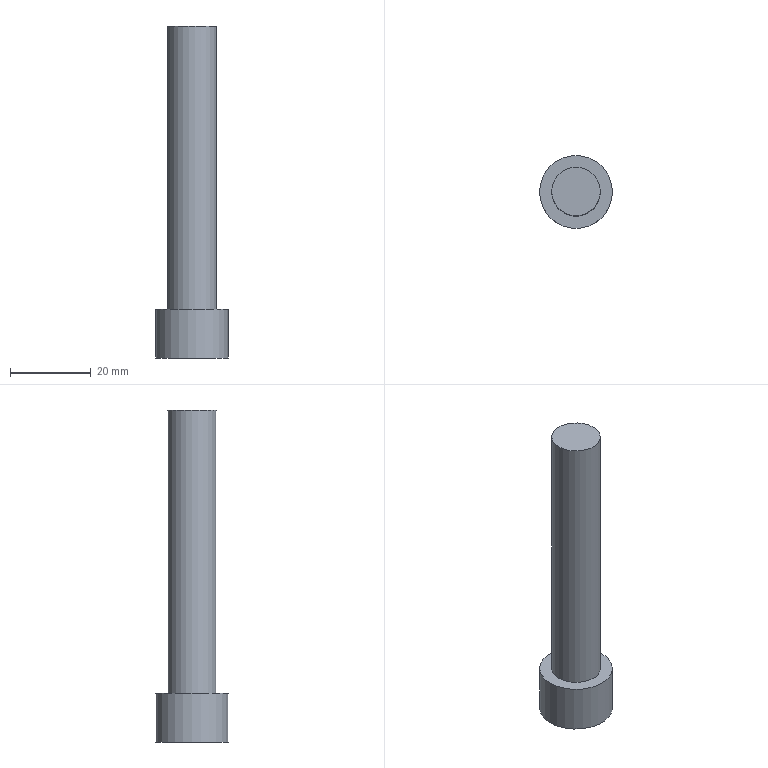Part | NX | features solid 2 | 1 solid | 12 faces | box 18 x 18 x 82 mm | volume 10451 mm3 | plane 10 | cylinder 2 | commonest cylinder face diameters 12 x1 18 x1
STEP:
#1=CARTESIAN_POINT('',(-264.,-305.,267.));
#2=VERTEX_POINT('',#1);
#3=CARTESIAN_POINT('',(-270.,-305.,267.));
#4=DIRECTION('',(0.,0.,1.));
#5=DIRECTION('',(1.,0.,0.));
#6=AXIS2_PLACEMENT_3D('',#3,#4,#5);
#7=CIRCLE('',#6,6.);
#8=EDGE_CURVE('',#2,#2,#7,.T.);
#9=ORIENTED_EDGE('',*,*,#8,.T.);
#10=EDGE_LOOP('',(#9));
#11=FACE_BOUND('',#10,.T.);
#12=CARTESIAN_POINT('',(-264.,-305.,337.));
#13=VERTEX_POINT('',#12);
#14=CARTESIAN_POINT('',(-270.,-305.,337.));
#15=DIRECTION('',(0.,0.,1.));
#16=DIRECTION('',(1.,0.,0.));
#17=AXIS2_PLACEMENT_3D('',#14,#15,#16);
#18=CIRCLE('',#17,6.);
#19=EDGE_CURVE('',#13,#13,#18,.T.);
#20=ORIENTED_EDGE('',*,*,#19,.F.);
#21=EDGE_LOOP('',(#20));
#22=FACE_BOUND('',#21,.T.);
#23=CARTESIAN_POINT('',(-270.,-305.,337.));
#24=DIRECTION('',(0.,0.,-1.));
#25=DIRECTION('',(-1.,0.,0.));
#26=AXIS2_PLACEMENT_3D('',#23,#24,#25);
#27=CYLINDRICAL_SURFACE('',#26,6.);
#28=ADVANCED_FACE('',(#11,#22),#27,.T.);
#29=ORIENTED_EDGE('',*,*,#19,.T.);
#30=EDGE_LOOP('',(#29));
#31=FACE_BOUND('',#30,.T.);
#32=CARTESIAN_POINT('',(-270.,-305.,337.));
#33=DIRECTION('',(0.,0.,1.));
#34=DIRECTION('',(1.,0.,0.));
#35=AXIS2_PLACEMENT_3D('',#32,#33,#34);
#36=PLANE('',#35);
#37=ADVANCED_FACE('',(#31),#36,.T.);
#38=CARTESIAN_POINT('',(-261.,-305.,267.));
#39=VERTEX_POINT('',#38);
#40=CARTESIAN_POINT('',(-270.,-305.,267.));
#41=DIRECTION('',(0.,0.,1.));
#42=DIRECTION('',(1.,0.,0.));
#43=AXIS2_PLACEMENT_3D('',#40,#41,#42);
#44=CIRCLE('',#43,9.);
#45=EDGE_CURVE('',#39,#39,#44,.T.);
#46=ORIENTED_EDGE('',*,*,#45,.T.);
#47=EDGE_LOOP('',(#46));
#48=FACE_BOUND('',#47,.T.);
#49=ORIENTED_EDGE('',*,*,#8,.F.);
#50=EDGE_LOOP('',(#49));
#51=FACE_BOUND('',#50,.T.);
#52=CARTESIAN_POINT('',(-270.,-305.,267.));
#53=DIRECTION('',(0.,0.,1.));
#54=DIRECTION('',(1.,0.,0.));
#55=AXIS2_PLACEMENT_3D('',#52,#53,#54);
#56=PLANE('',#55);
#57=ADVANCED_FACE('',(#48,#51),#56,.T.);
#58=CARTESIAN_POINT('',(-261.,-305.,255.));
#59=VERTEX_POINT('',#58);
#60=CARTESIAN_POINT('',(-270.,-305.,255.));
#61=DIRECTION('',(0.,0.,1.));
#62=DIRECTION('',(1.,0.,0.));
#63=AXIS2_PLACEMENT_3D('',#60,#61,#62);
#64=CIRCLE('',#63,9.);
#65=EDGE_CURVE('',#59,#59,#64,.T.);
#66=ORIENTED_EDGE('',*,*,#65,.T.);
#67=EDGE_LOOP('',(#66));
#68=FACE_BOUND('',#67,.T.);
#69=ORIENTED_EDGE('',*,*,#45,.F.);
#70=EDGE_LOOP('',(#69));
#71=FACE_BOUND('',#70,.T.);
#72=CARTESIAN_POINT('',(-270.,-305.,255.));
#73=DIRECTION('',(0.,0.,1.));
#74=DIRECTION('',(1.,0.,0.));
#75=AXIS2_PLACEMENT_3D('',#72,#73,#74);
#76=CYLINDRICAL_SURFACE('',#75,9.);
#77=ADVANCED_FACE('',(#68,#71),#76,.T.);
#78=CARTESIAN_POINT('',(-265.,-302.113,255.));
#79=VERTEX_POINT('',#78);
#80=CARTESIAN_POINT('',(-270.,-299.226,255.));
#81=VERTEX_POINT('',#80);
#82=CARTESIAN_POINT('',(-267.5,-300.67,255.));
#83=DIRECTION('',(-0.866,0.5,0.));
#84=VECTOR('',#83,1000.);
#85=LINE('',#82,#84);
#86=EDGE_CURVE('',#79,#81,#85,.T.);
#87=ORIENTED_EDGE('',*,*,#86,.T.);
#88=CARTESIAN_POINT('',(-275.,-302.113,255.));
#89=VERTEX_POINT('',#88);
#90=CARTESIAN_POINT('',(-272.5,-300.67,255.));
#91=DIRECTION('',(-0.866,-0.5,0.));
#92=VECTOR('',#91,1000.);
#93=LINE('',#90,#92);
#94=EDGE_CURVE('',#81,#89,#93,.T.);
#95=ORIENTED_EDGE('',*,*,#94,.T.);
#96=CARTESIAN_POINT('',(-275.,-307.887,255.));
#97=VERTEX_POINT('',#96);
#98=CARTESIAN_POINT('',(-275.,-305.,255.));
#99=DIRECTION('',(0.,-1.,0.));
#100=VECTOR('',#99,1000.);
#101=LINE('',#98,#100);
#102=EDGE_CURVE('',#89,#97,#101,.T.);
#103=ORIENTED_EDGE('',*,*,#102,.T.);
#104=CARTESIAN_POINT('',(-270.,-310.774,255.));
#105=VERTEX_POINT('',#104);
#106=CARTESIAN_POINT('',(-272.5,-309.33,255.));
#107=DIRECTION('',(0.866,-0.5,0.));
#108=VECTOR('',#107,1000.);
#109=LINE('',#106,#108);
#110=EDGE_CURVE('',#97,#105,#109,.T.);
#111=ORIENTED_EDGE('',*,*,#110,.T.);
#112=CARTESIAN_POINT('',(-265.,-307.887,255.));
#113=VERTEX_POINT('',#112);
#114=CARTESIAN_POINT('',(-267.5,-309.33,255.));
#115=DIRECTION('',(0.866,0.5,0.));
#116=VECTOR('',#115,1000.);
#117=LINE('',#114,#116);
#118=EDGE_CURVE('',#105,#113,#117,.T.);
#119=ORIENTED_EDGE('',*,*,#118,.T.);
#120=CARTESIAN_POINT('',(-265.,-305.,255.));
#121=DIRECTION('',(0.,1.,0.));
#122=VECTOR('',#121,1000.);
#123=LINE('',#120,#122);
#124=EDGE_CURVE('',#113,#79,#123,.T.);
#125=ORIENTED_EDGE('',*,*,#124,.T.);
#126=EDGE_LOOP('',(#87,#95,#103,#111,#119,#125));
#127=FACE_BOUND('',#126,.T.);
#128=ORIENTED_EDGE('',*,*,#65,.F.);
#129=EDGE_LOOP('',(#128));
#130=FACE_BOUND('',#129,.T.);
#131=CARTESIAN_POINT('',(-270.,-305.,255.));
#132=DIRECTION('',(0.,0.,1.));
#133=DIRECTION('',(1.,0.,0.));
#134=AXIS2_PLACEMENT_3D('',#131,#132,#133);
#135=PLANE('',#134);
#136=ADVANCED_FACE('',(#127,#130),#135,.F.);
#137=CARTESIAN_POINT('',(-270.,-299.226,261.));
#138=VERTEX_POINT('',#137);
#139=CARTESIAN_POINT('',(-270.,-299.226,241.));
#140=DIRECTION('',(0.,0.,1.));
#141=VECTOR('',#140,1000.);
#142=LINE('',#139,#141);
#143=EDGE_CURVE('',#81,#138,#142,.T.);
#144=ORIENTED_EDGE('',*,*,#143,.T.);
#145=CARTESIAN_POINT('',(-275.,-302.113,261.));
#146=VERTEX_POINT('',#145);
#147=CARTESIAN_POINT('',(-270.,-299.226,261.));
#148=DIRECTION('',(-0.866,-0.5,0.));
#149=VECTOR('',#148,1000.);
#150=LINE('',#147,#149);
#151=EDGE_CURVE('',#138,#146,#150,.T.);
#152=ORIENTED_EDGE('',*,*,#151,.T.);
#153=CARTESIAN_POINT('',(-275.,-302.113,241.));
#154=DIRECTION('',(0.,0.,1.));
#155=VECTOR('',#154,1000.);
#156=LINE('',#153,#155);
#157=EDGE_CURVE('',#89,#146,#156,.T.);
#158=ORIENTED_EDGE('',*,*,#157,.F.);
#159=ORIENTED_EDGE('',*,*,#94,.F.);
#160=EDGE_LOOP('',(#144,#152,#158,#159));
#161=FACE_BOUND('',#160,.T.);
#162=CARTESIAN_POINT('',(-270.,-299.226,241.));
#163=DIRECTION('',(-0.5,0.866,0.));
#164=DIRECTION('',(-0.866,-0.5,0.));
#165=AXIS2_PLACEMENT_3D('',#162,#163,#164);
#166=PLANE('',#165);
#167=ADVANCED_FACE('',(#161),#166,.F.);
#168=ORIENTED_EDGE('',*,*,#157,.T.);
#169=CARTESIAN_POINT('',(-275.,-307.887,261.));
#170=VERTEX_POINT('',#169);
#171=CARTESIAN_POINT('',(-275.,-302.113,261.));
#172=DIRECTION('',(0.,-1.,0.));
#173=VECTOR('',#172,1000.);
#174=LINE('',#171,#173);
#175=EDGE_CURVE('',#146,#170,#174,.T.);
#176=ORIENTED_EDGE('',*,*,#175,.T.);
#177=CARTESIAN_POINT('',(-275.,-307.887,241.));
#178=DIRECTION('',(0.,0.,1.));
#179=VECTOR('',#178,1000.);
#180=LINE('',#177,#179);
#181=EDGE_CURVE('',#97,#170,#180,.T.);
#182=ORIENTED_EDGE('',*,*,#181,.F.);
#183=ORIENTED_EDGE('',*,*,#102,.F.);
#184=EDGE_LOOP('',(#168,#176,#182,#183));
#185=FACE_BOUND('',#184,.T.);
#186=CARTESIAN_POINT('',(-275.,-302.113,241.));
#187=DIRECTION('',(-1.,0.,0.));
#188=DIRECTION('',(0.,0.,1.));
#189=AXIS2_PLACEMENT_3D('',#186,#187,#188);
#190=PLANE('',#189);
#191=ADVANCED_FACE('',(#185),#190,.F.);
#192=ORIENTED_EDGE('',*,*,#181,.T.);
#193=CARTESIAN_POINT('',(-270.,-310.774,261.));
#194=VERTEX_POINT('',#193);
#195=CARTESIAN_POINT('',(-275.,-307.887,261.));
#196=DIRECTION('',(0.866,-0.5,0.));
#197=VECTOR('',#196,1000.);
#198=LINE('',#195,#197);
#199=EDGE_CURVE('',#170,#194,#198,.T.);
#200=ORIENTED_EDGE('',*,*,#199,.T.);
#201=CARTESIAN_POINT('',(-270.,-310.774,241.));
#202=DIRECTION('',(0.,0.,1.));
#203=VECTOR('',#202,1000.);
#204=LINE('',#201,#203);
#205=EDGE_CURVE('',#105,#194,#204,.T.);
#206=ORIENTED_EDGE('',*,*,#205,.F.);
#207=ORIENTED_EDGE('',*,*,#110,.F.);
#208=EDGE_LOOP('',(#192,#200,#206,#207));
#209=FACE_BOUND('',#208,.T.);
#210=CARTESIAN_POINT('',(-275.,-307.887,241.));
#211=DIRECTION('',(-0.5,-0.866,0.));
#212=DIRECTION('',(0.866,-0.5,0.));
#213=AXIS2_PLACEMENT_3D('',#210,#211,#212);
#214=PLANE('',#213);
#215=ADVANCED_FACE('',(#209),#214,.F.);
#216=ORIENTED_EDGE('',*,*,#205,.T.);
#217=CARTESIAN_POINT('',(-265.,-307.887,261.));
#218=VERTEX_POINT('',#217);
#219=CARTESIAN_POINT('',(-270.,-310.774,261.));
#220=DIRECTION('',(0.866,0.5,0.));
#221=VECTOR('',#220,1000.);
#222=LINE('',#219,#221);
#223=EDGE_CURVE('',#194,#218,#222,.T.);
#224=ORIENTED_EDGE('',*,*,#223,.T.);
#225=CARTESIAN_POINT('',(-265.,-307.887,241.));
#226=DIRECTION('',(0.,0.,1.));
#227=VECTOR('',#226,1000.);
#228=LINE('',#225,#227);
#229=EDGE_CURVE('',#113,#218,#228,.T.);
#230=ORIENTED_EDGE('',*,*,#229,.F.);
#231=ORIENTED_EDGE('',*,*,#118,.F.);
#232=EDGE_LOOP('',(#216,#224,#230,#231));
#233=FACE_BOUND('',#232,.T.);
#234=CARTESIAN_POINT('',(-270.,-310.774,241.));
#235=DIRECTION('',(0.5,-0.866,0.));
#236=DIRECTION('',(0.866,0.5,0.));
#237=AXIS2_PLACEMENT_3D('',#234,#235,#236);
#238=PLANE('',#237);
#239=ADVANCED_FACE('',(#233),#238,.F.);
#240=ORIENTED_EDGE('',*,*,#229,.T.);
#241=CARTESIAN_POINT('',(-265.,-302.113,261.));
#242=VERTEX_POINT('',#241);
#243=CARTESIAN_POINT('',(-265.,-307.887,261.));
#244=DIRECTION('',(0.,1.,0.));
#245=VECTOR('',#244,1000.);
#246=LINE('',#243,#245);
#247=EDGE_CURVE('',#218,#242,#246,.T.);
#248=ORIENTED_EDGE('',*,*,#247,.T.);
#249=CARTESIAN_POINT('',(-265.,-302.113,241.));
#250=DIRECTION('',(0.,0.,1.));
#251=VECTOR('',#250,1000.);
#252=LINE('',#249,#251);
#253=EDGE_CURVE('',#79,#242,#252,.T.);
#254=ORIENTED_EDGE('',*,*,#253,.F.);
#255=ORIENTED_EDGE('',*,*,#124,.F.);
#256=EDGE_LOOP('',(#240,#248,#254,#255));
#257=FACE_BOUND('',#256,.T.);
#258=CARTESIAN_POINT('',(-265.,-307.887,241.));
#259=DIRECTION('',(1.,0.,0.));
#260=DIRECTION('',(0.,0.,-1.));
#261=AXIS2_PLACEMENT_3D('',#258,#259,#260);
#262=PLANE('',#261);
#263=ADVANCED_FACE('',(#257),#262,.F.);
#264=ORIENTED_EDGE('',*,*,#253,.T.);
#265=CARTESIAN_POINT('',(-265.,-302.113,261.));
#266=DIRECTION('',(-0.866,0.5,0.));
#267=VECTOR('',#266,1000.);
#268=LINE('',#265,#267);
#269=EDGE_CURVE('',#242,#138,#268,.T.);
#270=ORIENTED_EDGE('',*,*,#269,.T.);
#271=ORIENTED_EDGE('',*,*,#143,.F.);
#272=ORIENTED_EDGE('',*,*,#86,.F.);
#273=EDGE_LOOP('',(#264,#270,#271,#272));
#274=FACE_BOUND('',#273,.T.);
#275=CARTESIAN_POINT('',(-265.,-302.113,241.));
#276=DIRECTION('',(0.5,0.866,0.));
#277=DIRECTION('',(-0.866,0.5,0.));
#278=AXIS2_PLACEMENT_3D('',#275,#276,#277);
#279=PLANE('',#278);
#280=ADVANCED_FACE('',(#274),#279,.F.);
#281=ORIENTED_EDGE('',*,*,#151,.F.);
#282=ORIENTED_EDGE('',*,*,#269,.F.);
#283=ORIENTED_EDGE('',*,*,#247,.F.);
#284=ORIENTED_EDGE('',*,*,#223,.F.);
#285=ORIENTED_EDGE('',*,*,#199,.F.);
#286=ORIENTED_EDGE('',*,*,#175,.F.);
#287=EDGE_LOOP('',(#281,#282,#283,#284,#285,#286));
#288=FACE_BOUND('',#287,.T.);
#289=CARTESIAN_POINT('',(-280.,-305.,261.));
#290=DIRECTION('',(0.,0.,1.));
#291=DIRECTION('',(1.,0.,0.));
#292=AXIS2_PLACEMENT_3D('',#289,#290,#291);
#293=PLANE('',#292);
#294=ADVANCED_FACE('',(#288),#293,.F.);
#295=CLOSED_SHELL('',(#28,#37,#57,#77,#136,#167,#191,#215,#239,#263,#280,#294));
#296=MANIFOLD_SOLID_BREP('',#295);
#297=(LENGTH_UNIT()NAMED_UNIT(*)SI_UNIT(.MILLI.,.METRE.));
#298=UNCERTAINTY_MEASURE_WITH_UNIT(LENGTH_MEASURE(0.00001),#297,'','');
#299=(NAMED_UNIT(*)PLANE_ANGLE_UNIT()SI_UNIT($,.RADIAN.));
#300=(NAMED_UNIT(*)SI_UNIT($,.STERADIAN.)SOLID_ANGLE_UNIT());
#301=(GEOMETRIC_REPRESENTATION_CONTEXT(3)GLOBAL_UNCERTAINTY_ASSIGNED_CONTEXT((#298))GLOBAL_UNIT_ASSIGNED_CONTEXT((#297,#299,#300))REPRESENTATION_CONTEXT('',''));
#302=ADVANCED_BREP_SHAPE_REPRESENTATION('',(#296),#301);